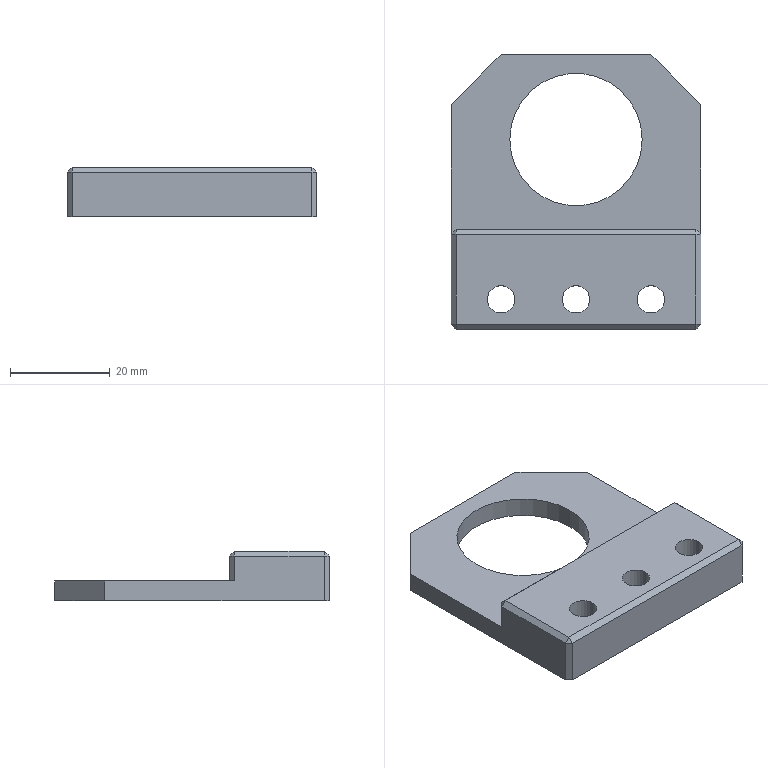Part | STEP file | BPSP-11-10 Pusher Cylinder Fixing Plate_Default | 1 solid | 30 faces | box 50 x 55 x 10 mm | volume 13598 mm3 | plane 22 | cylinder 8 | commonest cylinder face diameters 5.5 x6 26.5 x2